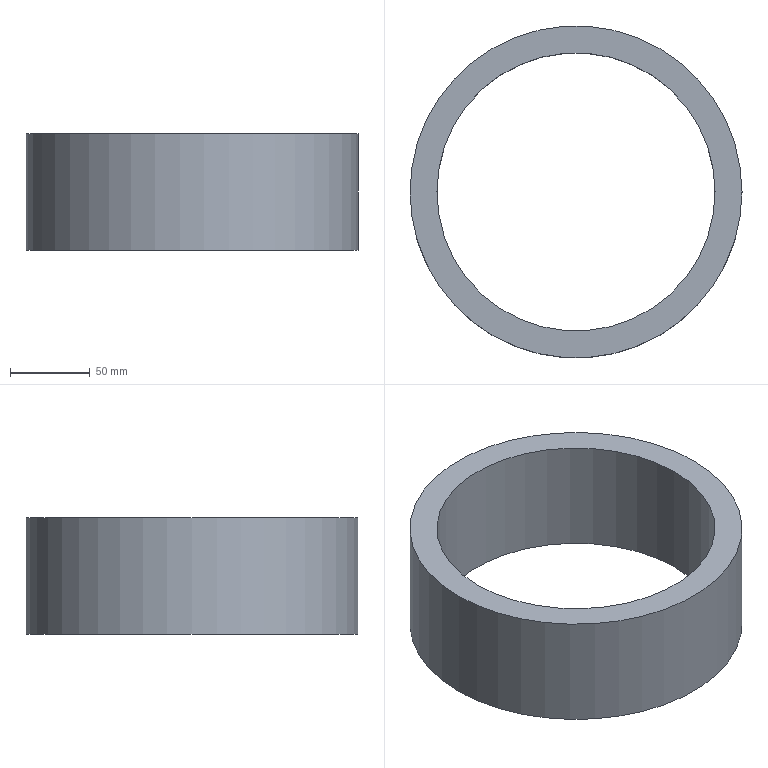Part | NX | features CYLINDER 2, DATUM_CSYS 1, Delete Body 1, LINKED_BODY 1, SCALE 1 | 1 solid | 4 faces | box 208.125 x 208.125 x 73.125 mm | volume 741414 mm3 | plane 2 | cylinder 2 | commonest cylinder face diameters 174.375 x1 208.125 x1
STEP:
#1=CARTESIAN_POINT('',(-453.77,-1724.979,-13.875));
#2=VERTEX_POINT('',#1);
#3=CARTESIAN_POINT('',(-366.582,-1724.979,-13.875));
#4=DIRECTION('',(0.,0.,-1.));
#5=DIRECTION('',(-1.,0.,0.));
#6=AXIS2_PLACEMENT_3D('',#3,#4,#5);
#7=CIRCLE('',#6,87.188);
#8=EDGE_CURVE('',#2,#2,#7,.T.);
#9=ORIENTED_EDGE('',*,*,#8,.T.);
#10=EDGE_LOOP('',(#9));
#11=FACE_BOUND('',#10,.T.);
#12=CARTESIAN_POINT('',(-470.645,-1724.979,-13.875));
#13=VERTEX_POINT('',#12);
#14=CARTESIAN_POINT('',(-366.582,-1724.979,-13.875));
#15=DIRECTION('',(0.,0.,-1.));
#16=DIRECTION('',(-1.,0.,0.));
#17=AXIS2_PLACEMENT_3D('',#14,#15,#16);
#18=CIRCLE('',#17,104.062);
#19=EDGE_CURVE('',#13,#13,#18,.T.);
#20=ORIENTED_EDGE('',*,*,#19,.F.);
#21=EDGE_LOOP('',(#20));
#22=FACE_BOUND('',#21,.T.);
#23=CARTESIAN_POINT('',(-366.582,-1724.979,-13.875));
#24=DIRECTION('',(0.,0.,1.));
#25=DIRECTION('',(1.,0.,0.));
#26=AXIS2_PLACEMENT_3D('',#23,#24,#25);
#27=PLANE('',#26);
#28=ADVANCED_FACE('',(#11,#22),#27,.T.);
#29=CARTESIAN_POINT('',(-279.395,-1724.979,-87.));
#30=VERTEX_POINT('',#29);
#31=CARTESIAN_POINT('',(-366.582,-1724.979,-87.));
#32=DIRECTION('',(0.,0.,1.));
#33=DIRECTION('',(1.,0.,0.));
#34=AXIS2_PLACEMENT_3D('',#31,#32,#33);
#35=CIRCLE('',#34,87.188);
#36=EDGE_CURVE('',#30,#30,#35,.T.);
#37=ORIENTED_EDGE('',*,*,#36,.T.);
#38=EDGE_LOOP('',(#37));
#39=FACE_BOUND('',#38,.T.);
#40=CARTESIAN_POINT('',(-262.52,-1724.979,-87.));
#41=VERTEX_POINT('',#40);
#42=CARTESIAN_POINT('',(-366.582,-1724.979,-87.));
#43=DIRECTION('',(0.,0.,1.));
#44=DIRECTION('',(1.,0.,0.));
#45=AXIS2_PLACEMENT_3D('',#42,#43,#44);
#46=CIRCLE('',#45,104.062);
#47=EDGE_CURVE('',#41,#41,#46,.T.);
#48=ORIENTED_EDGE('',*,*,#47,.F.);
#49=EDGE_LOOP('',(#48));
#50=FACE_BOUND('',#49,.T.);
#51=CARTESIAN_POINT('',(-366.582,-1724.979,-87.));
#52=DIRECTION('',(0.,0.,-1.));
#53=DIRECTION('',(-1.,0.,0.));
#54=AXIS2_PLACEMENT_3D('',#51,#52,#53);
#55=PLANE('',#54);
#56=ADVANCED_FACE('',(#39,#50),#55,.T.);
#57=ORIENTED_EDGE('',*,*,#19,.T.);
#58=EDGE_LOOP('',(#57));
#59=FACE_BOUND('',#58,.T.);
#60=ORIENTED_EDGE('',*,*,#47,.T.);
#61=EDGE_LOOP('',(#60));
#62=FACE_BOUND('',#61,.T.);
#63=CARTESIAN_POINT('',(-366.582,-1724.979,-87.));
#64=DIRECTION('',(0.,0.,1.));
#65=DIRECTION('',(1.,0.,0.));
#66=AXIS2_PLACEMENT_3D('',#63,#64,#65);
#67=CYLINDRICAL_SURFACE('',#66,104.062);
#68=ADVANCED_FACE('',(#59,#62),#67,.T.);
#69=ORIENTED_EDGE('',*,*,#8,.F.);
#70=EDGE_LOOP('',(#69));
#71=FACE_BOUND('',#70,.T.);
#72=ORIENTED_EDGE('',*,*,#36,.F.);
#73=EDGE_LOOP('',(#72));
#74=FACE_BOUND('',#73,.T.);
#75=CARTESIAN_POINT('',(-366.582,-1724.979,-87.));
#76=DIRECTION('',(0.,0.,1.));
#77=DIRECTION('',(1.,0.,0.));
#78=AXIS2_PLACEMENT_3D('',#75,#76,#77);
#79=CYLINDRICAL_SURFACE('',#78,87.188);
#80=ADVANCED_FACE('',(#71,#74),#79,.F.);
#81=CLOSED_SHELL('',(#28,#56,#68,#80));
#82=MANIFOLD_SOLID_BREP('',#81);
#83=(LENGTH_UNIT()NAMED_UNIT(*)SI_UNIT(.MILLI.,.METRE.));
#84=UNCERTAINTY_MEASURE_WITH_UNIT(LENGTH_MEASURE(0.00001),#83,'','');
#85=(NAMED_UNIT(*)PLANE_ANGLE_UNIT()SI_UNIT($,.RADIAN.));
#86=(NAMED_UNIT(*)SI_UNIT($,.STERADIAN.)SOLID_ANGLE_UNIT());
#87=(GEOMETRIC_REPRESENTATION_CONTEXT(3)GLOBAL_UNCERTAINTY_ASSIGNED_CONTEXT((#84))GLOBAL_UNIT_ASSIGNED_CONTEXT((#83,#85,#86))REPRESENTATION_CONTEXT('',''));
#88=ADVANCED_BREP_SHAPE_REPRESENTATION('',(#82),#87);